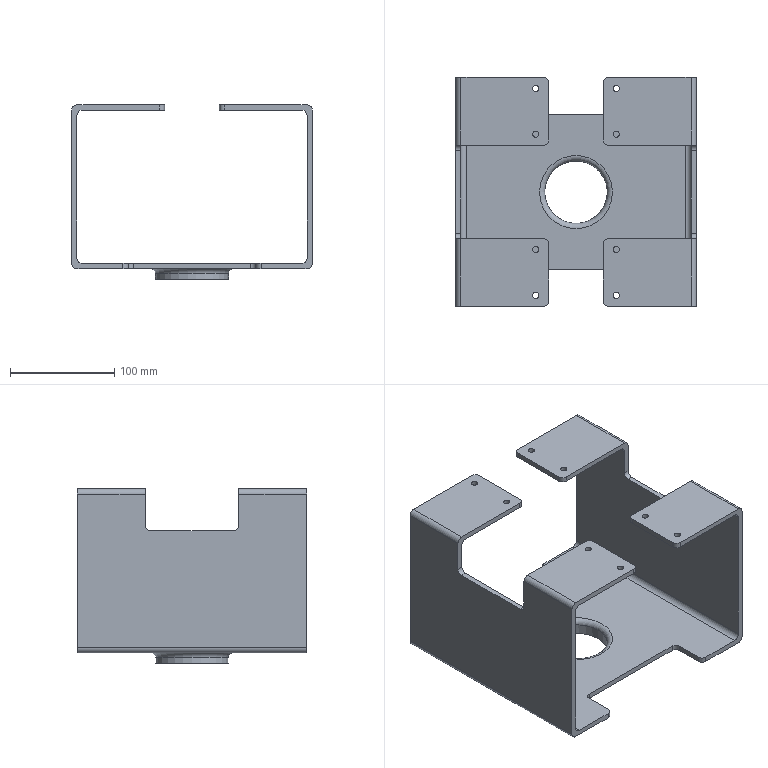Part | NX | features BREP 1 | 1 solid | 79 faces | box 230.462 x 219.464 x 166.967 mm | volume 611009 mm3 | cylinder 42 | plane 35 | torus 2 | commonest cylinder face diameters 10 x32 6 x8 60 x1 70 x1